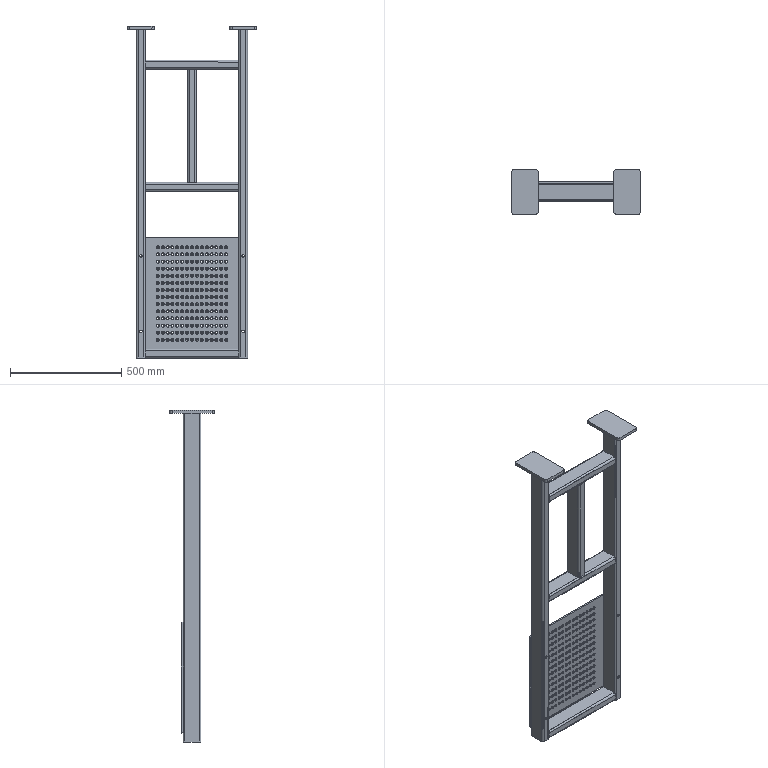Part | SolidWorks | 9 solids | 1430 faces | box 580 x 200 x 1494 mm | volume 6577657 mm3 | torus 840 | cylinder 504 | plane 86 | commonest cylinder face diameters 8 x444 16 x28 12 x24 20 x8